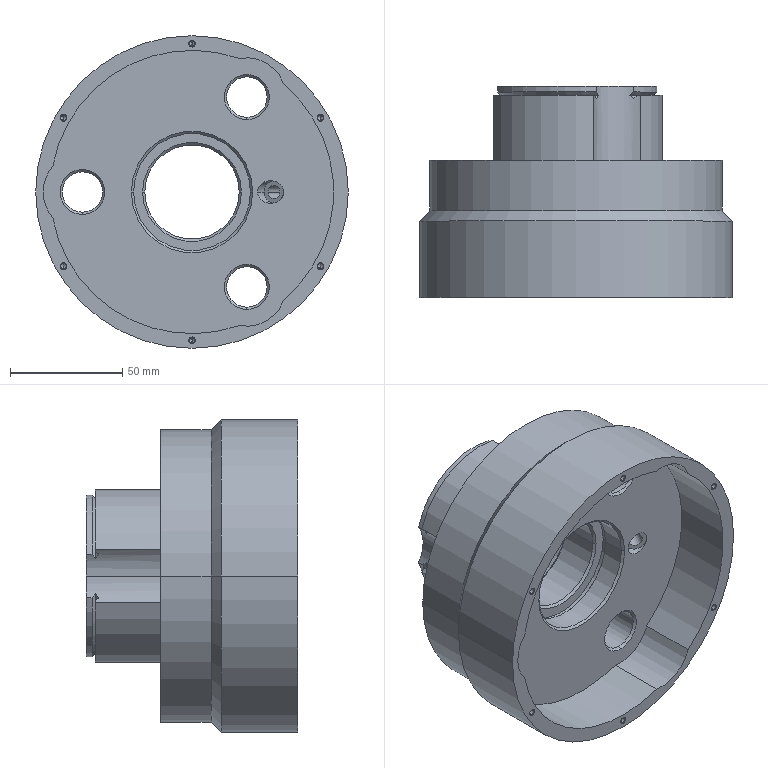Part | SolidWorks | features Chamfer 3, ICE 3, CirPattern 2, RevCut 2, SweepCut 2, HoleWzd 1, Revolution 1 | 1 solid | 125 faces | box 139 x 94 x 139 mm | volume 531526 mm3 | cone 58 | cylinder 55 | plane 12 | commonest cylinder face diameters 2.5 x12 18 x6 6 x4 34 x4 35 x4 52 x4